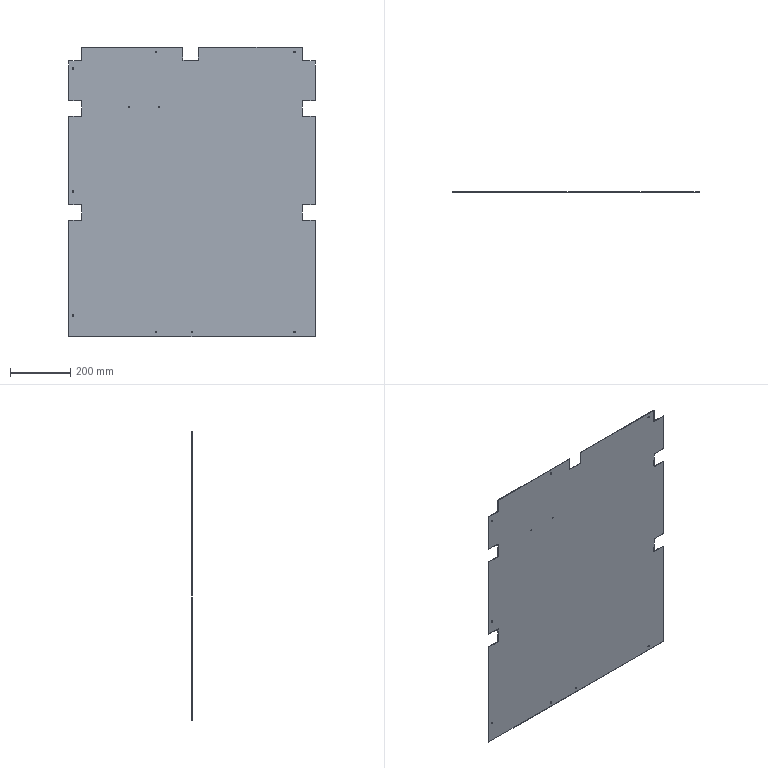Part | NX | features BREP 1 | 1 solid | 50 faces | box 821 x 1.5 x 963.5 mm | volume 1163682 mm3 | plane 30 | cylinder 20 | commonest cylinder face diameters 5 x16 3.3 x4